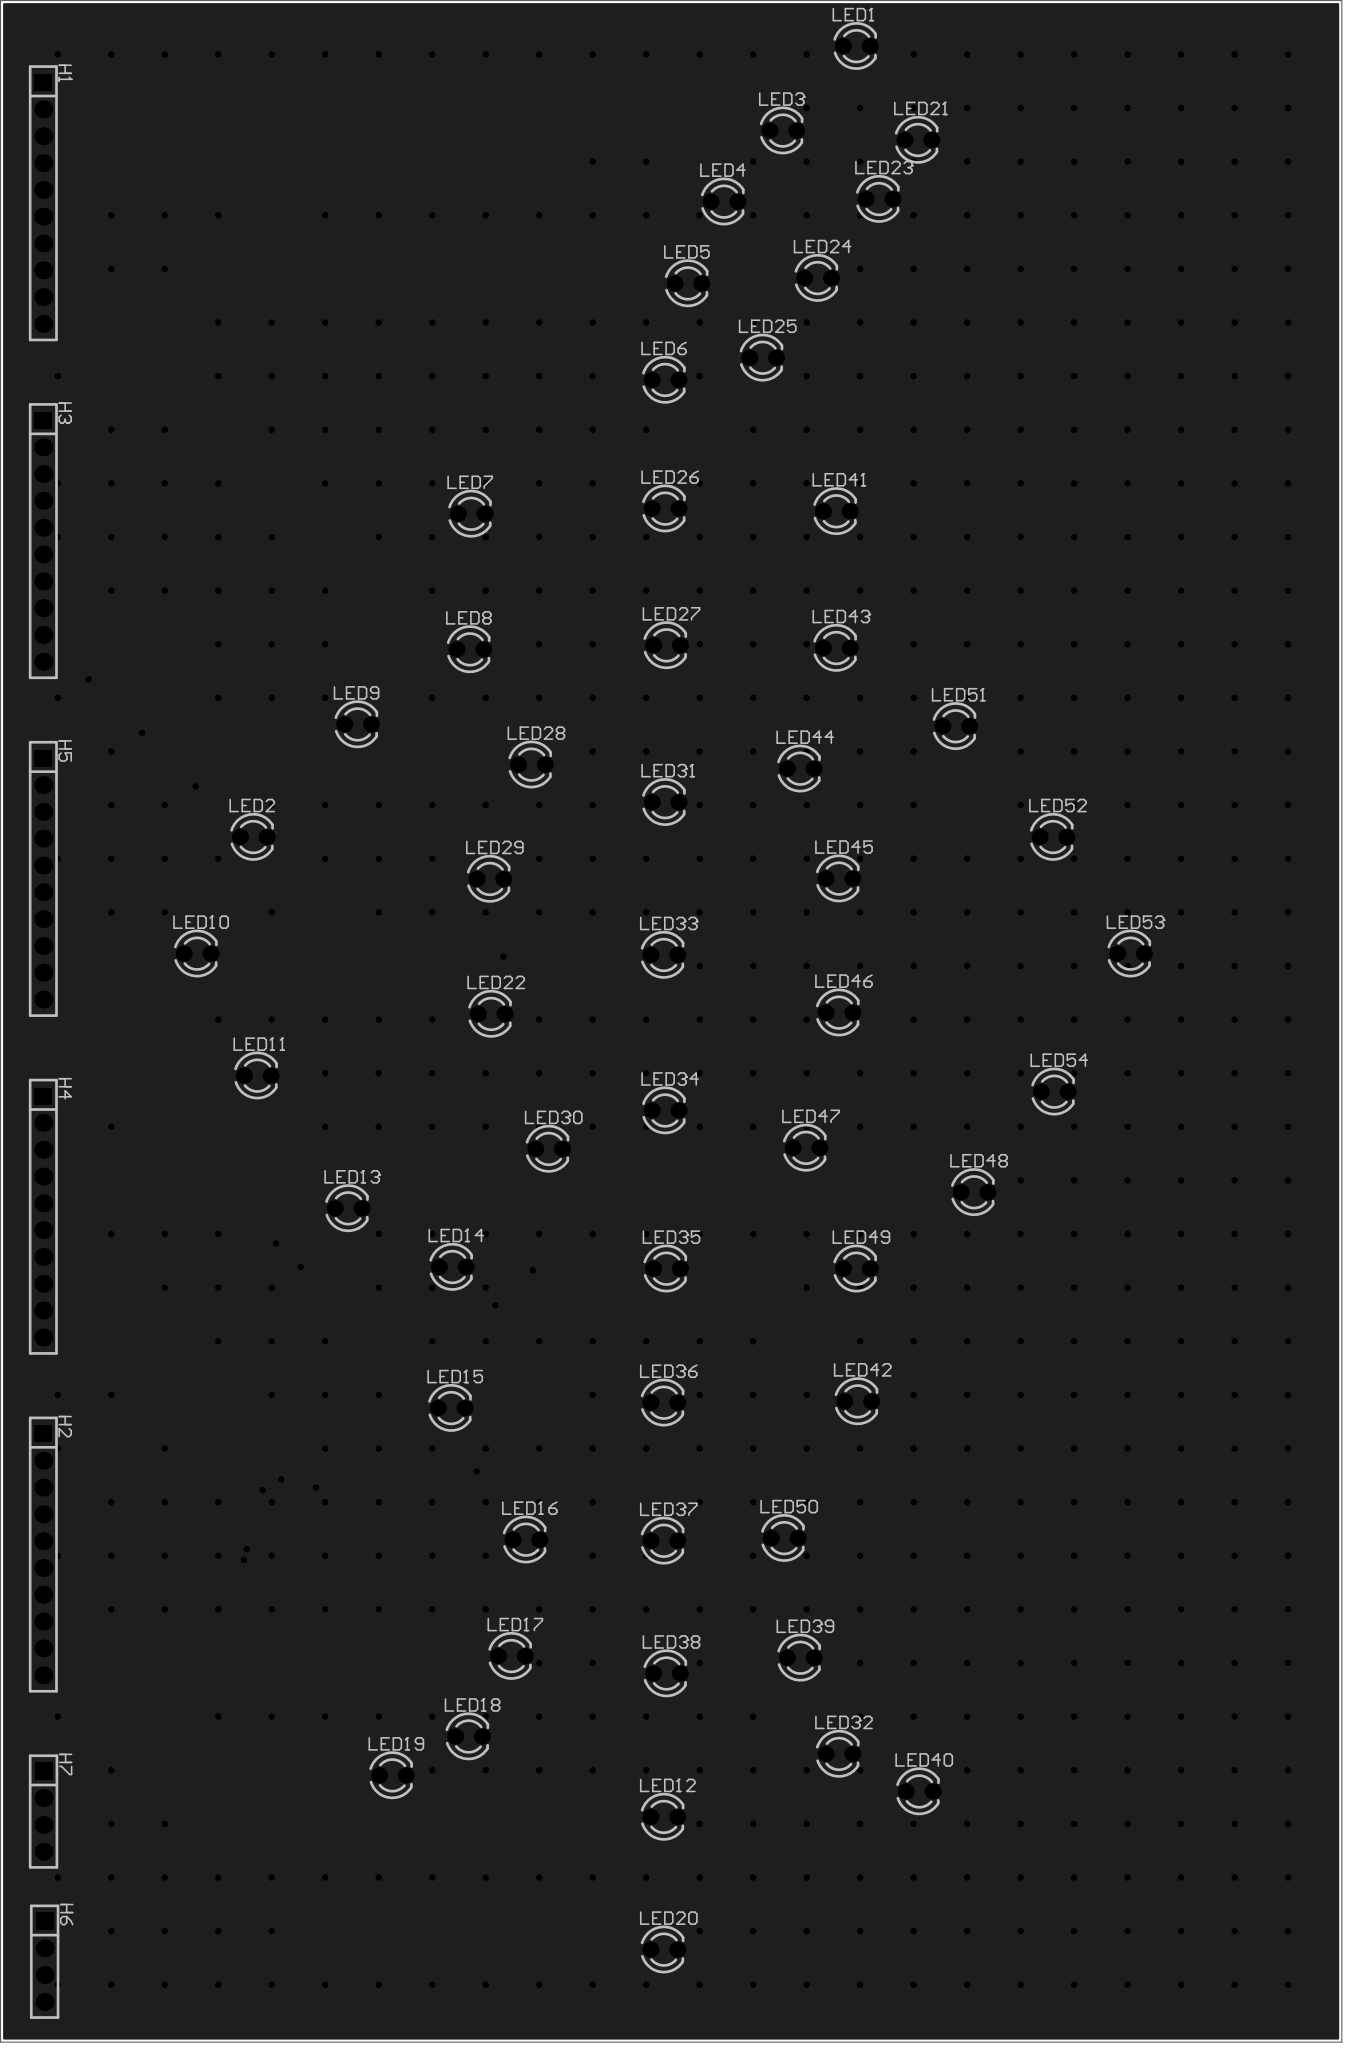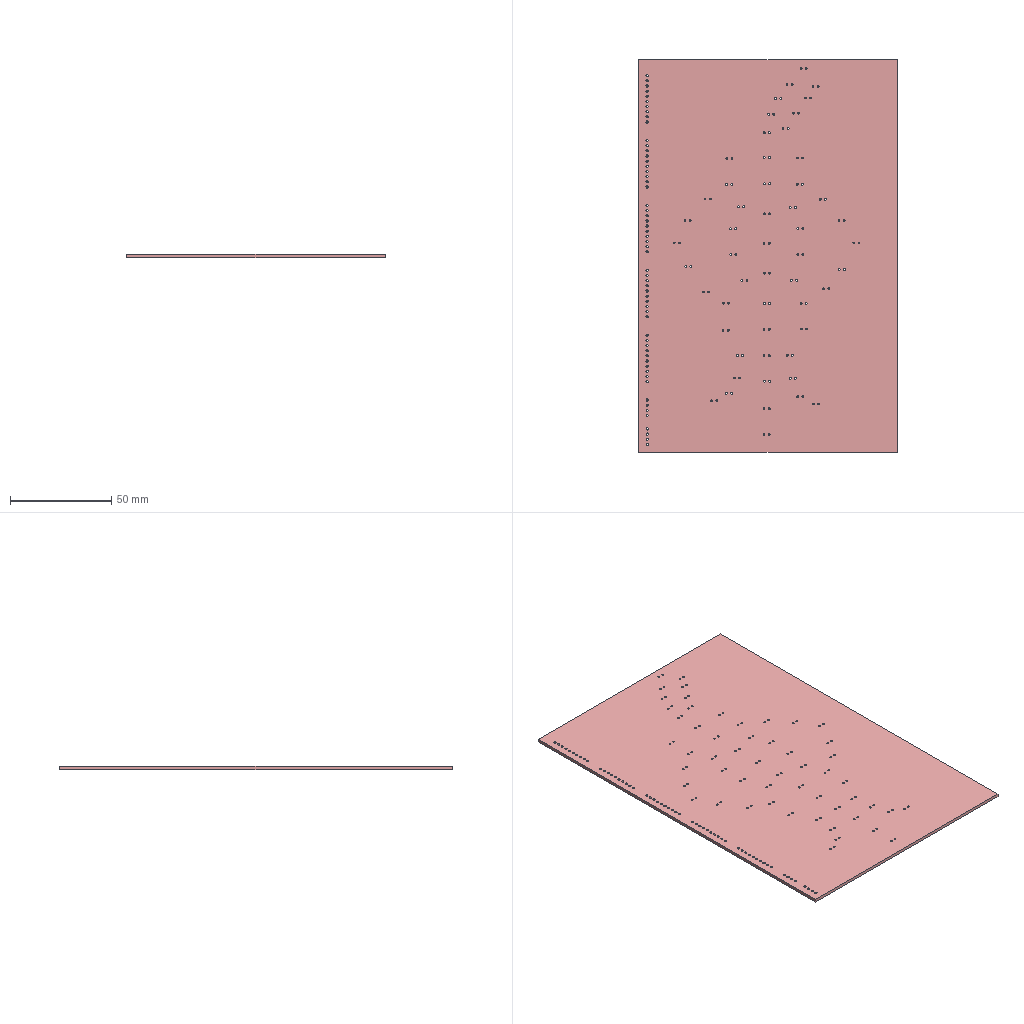Circuit board layout | Altium Designer | box 127.4 x 193.4 x 1.6 mm
Layer stack:
# Altium Designer layer stack of  (unit mm; dielectric type: 0 none, 1 core, 2 prepreg, 3 surface material)
index,name,kind,layer,copper_thickness_mm,dielectric_type,dielectric_thickness_mm,dielectric_material,dielectric_constant
0,Top Paste Mask Layer,other,,,,,,
1,Top Silkscreen Layer,other,,,,,,
2,Top Solder Mask Layer,dielectric,,,3,0.01,,3.3
3,Top Layer,copper,Top Layer,0.035,,,,
4,Dielectric1,dielectric,,,3,1.51,FR4,4.5
5,Bottom Layer,copper,Bottom Layer,0.035,,,,
6,Bottom Solder Mask Layer,dielectric,,,3,0.01,,3.3
7,Bottom Silkscreen Layer,other,,,,,,
8,Bottom Paste Mask Layer,other,,,,,,
# drill layer pairs: low layer,high layer
drill_pair,Top Layer,Bottom Layer
Part placement:
Designator,Comment,Layer,Footprint,Center-X(mm),Center-Y(mm),Rotation
H1,,TopLayer,HDR-TH_10P-P2.54-V-F,112.776,270.737,270
H2,,TopLayer,HDR-TH_10P-P2.54-V-F,112.776,142.711,270
H3,,TopLayer,HDR-TH_10P-P2.54-V-F,112.776,238.73,270
H4,,TopLayer,HDR-TH_10P-P2.54-V-F,112.776,174.717,270
H5,,TopLayer,HDR-TH_10P-P2.54-V-F,112.776,206.724,270
H6,,TopLayer,HDR-TH_4P-P2.54-V-F,112.903,104.14,270
LED1,,TopLayer,LED_TH-3mm,189.992,285.623,0
LED2,,TopLayer,LED_TH-3mm,132.715,210.693,0
LED3,,TopLayer,LED_TH-3mm,183.007,277.622,0
LED4,,TopLayer,LED_TH-3mm,177.419,270.891,0
LED5,,TopLayer,LED_TH-3mm,173.99,263.144,0
LED6,,TopLayer,LED_TH-3mm,171.831,254,0
LED7,,TopLayer,LED_TH-3mm,153.412,241.316,0
LED8,,TopLayer,LED_TH-3mm,153.289,228.473,0
LED9,,TopLayer,LED_TH-3mm,142.621,221.361,0
LED10,,TopLayer,LED_TH-3mm,127.381,199.644,0
LED11,,TopLayer,LED_TH-3mm,133.096,188.087,0
LED12,,TopLayer,LED_TH-3mm,171.704,117.856,0
LED13,,TopLayer,LED_TH-3mm,141.732,175.514,0
LED14,,TopLayer,LED_TH-3mm,151.622,169.955,0
LED15,,TopLayer,LED_TH-3mm,151.511,156.591,0
LED16,,TopLayer,LED_TH-3mm,158.607,144.123,0
LED17,,TopLayer,LED_TH-3mm,157.226,133.096,0
LED18,,TopLayer,LED_TH-3mm,153.162,125.476,0
LED19,,TopLayer,LED_TH-3mm,145.923,121.793,0
LED20,,TopLayer,LED_TH-3mm,171.704,105.283,0
LED21,,TopLayer,LED_TH-3mm,195.834,276.733,0
LED22,,TopLayer,LED_TH-3mm,155.313,193.933,0
LED23,,TopLayer,LED_TH-3mm,192.143,271.136,0
LED24,,TopLayer,LED_TH-3mm,186.309,263.652,0
LED25,,TopLayer,LED_TH-3mm,181.094,256.099,0
LED26,,TopLayer,LED_TH-3mm,171.831,241.808,0
LED27,,TopLayer,LED_TH-3mm,171.958,228.854,0
LED28,,TopLayer,LED_TH-3mm,159.131,217.551,0
LED29,,TopLayer,LED_TH-3mm,155.186,206.722,0
LED30,,TopLayer,LED_TH-3mm,160.774,181.144,0
LED31,,TopLayer,LED_TH-3mm,171.831,213.995,0
LED32,,TopLayer,LED_TH-3mm,188.341,123.825,0
LED33,,TopLayer,LED_TH-3mm,171.704,199.517,0
LED34,,TopLayer,LED_TH-3mm,171.831,184.785,0
LED35,,TopLayer,LED_TH-3mm,171.958,169.799,0
LED36,,TopLayer,LED_TH-3mm,171.704,157.099,0
LED37,,TopLayer,LED_TH-3mm,171.704,144.018,0
LED38,,TopLayer,LED_TH-3mm,171.958,131.445,0
LED39,,TopLayer,LED_TH-3mm,184.674,132.935,0
LED40,,TopLayer,LED_TH-3mm,195.961,120.269,0
LED41,,TopLayer,LED_TH-3mm,188.087,241.554,0
LED42,,TopLayer,LED_TH-3mm,190.119,157.226,0
LED43,,TopLayer,LED_TH-3mm,188.087,228.6,0
LED44,,TopLayer,LED_TH-3mm,184.658,217.17,0
LED45,,TopLayer,LED_TH-3mm,188.341,206.756,0
LED46,,TopLayer,LED_TH-3mm,188.341,194.056,0
LED47,,TopLayer,LED_TH-3mm,185.206,181.245,0
LED48,,TopLayer,LED_TH-3mm,201.168,177.038,0
LED49,,TopLayer,LED_TH-3mm,189.992,169.799,0
LED50,,TopLayer,LED_TH-3mm,183.134,144.272,0
H7,,TopLayer,HDR-TH_4P-P2.54-V-F,112.796,118.364,270
LED51,,TopLayer,LED_TH-3mm,199.422,221.189,0
LED52,,TopLayer,LED_TH-3mm,208.661,210.693,0
LED53,,TopLayer,LED_TH-3mm,216.027,199.644,0
LED54,,TopLayer,LED_TH-3mm,208.788,186.563,0
Pad and via stacks:
# Altium Designer via and pad stacks of  (unit mm). Each distinct definition once, with the count of objects using it.
# via: kind,start_layer,end_layer,hole_mm,diameter_mm,mode(0 simple;1 top-mid-bottom;2 full stack),diameter_per_layer,count,example_net
# pad: kind,layer,hole_mm,hole_type(0 round;1 square;2 slot),plating,top_size,top_shape(1 round;2 rect;3 octagon;9 rounded rect),mid_size,bottom_size,mode,footprint,size_per_layer,count,example
pad,Multi-Layer,1.1,0,plated,1.7x1.7,1,1.7x1.7,1.7x1.7,0,HDR-TH_10P-P2.54-V-F,,45,H1.10
pad,Multi-Layer,1.1,0,plated,1.575x1.7,2,1.575x1.7,1.575x1.7,0,HDR-TH_10P-P2.54-V-F,,5,H1.1
pad,Multi-Layer,1.1,0,plated,1.7x1.7,2,1.7x1.7,1.7x1.7,0,HDR-TH_4P-P2.54-V-F,,2,H6.1
pad,Multi-Layer,1.1,0,plated,1.7x1.7,1,1.7x1.7,1.7x1.7,0,HDR-TH_4P-P2.54-V-F,,6,H6.2
pad,Multi-Layer,0.9144,0,plated,1.524x1.524,1,1.524x1.524,1.524x1.524,0,LED_TH-3mm,,108,LED1.1
via,Top Layer,Bottom Layer,0.3048,0.61,0,,702,P54
Copper pours:
name,layer,net,type(0 solid;1 hatched;2 none)
Top Layer-VCC,Top Layer,VCC,0
Bottom Layer-VCC,Bottom Layer,VCC,0
Design rules, without the lines most boards share:
# Altium Designer design rules of  (exported by Altium Designer, unit mm)
# columns: name | kind | enabled | priority | scope1 | scope2 | descriptor | typed fields (field=value)
creepage | 65 | enabled | 1 | All | All | Creepage Distance Constraint =(0mil) (All),(All) |
copperRegion | 20 | enabled | 1 | (InNet('P18') OR InNet('P19')) | All | Polygon Connect Rule(Relief Connect )(Conductor Width=10mil) (Relief Angle=90 Angle) (Entries=4) (Air Gap Width=10mil) ((InNet('P18') OR InNet('P19'))),(All) | connect_style(0=relief,1=direct,2=none)=0 relief_conductor_width=0.254 relief_entries=4